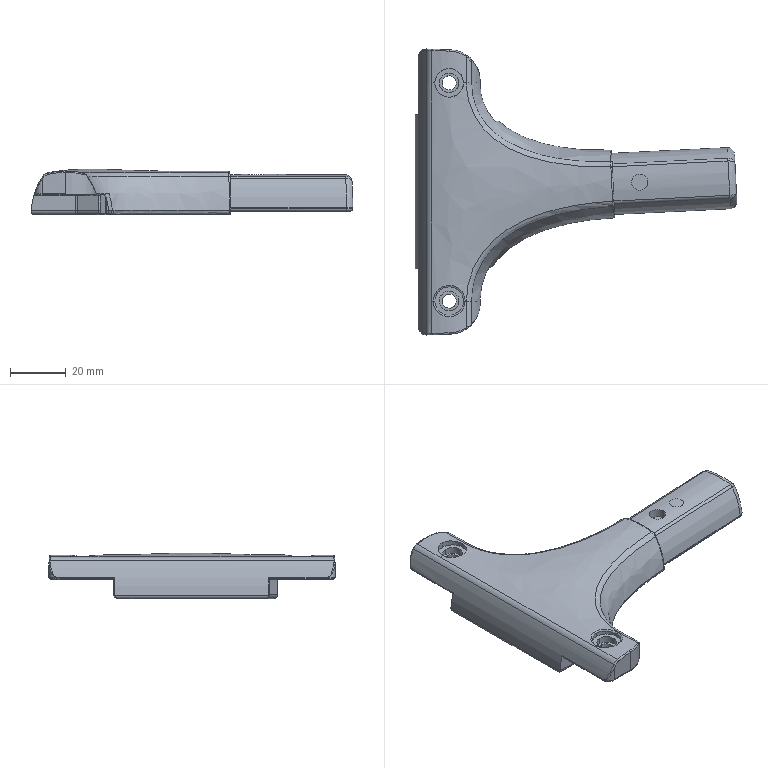Part | SolidWorks | features BaseBody 1 | 1 solid | 551 faces | box 115.648 x 102.814 x 16.383 mm | volume 42837 mm3 | plane 275 | spline 145 | cylinder 131 | commonest cylinder face diameters 2.745 x19 0.98 x11 5.882 x10 41.765 x10 2.941 x6 5.098 x6